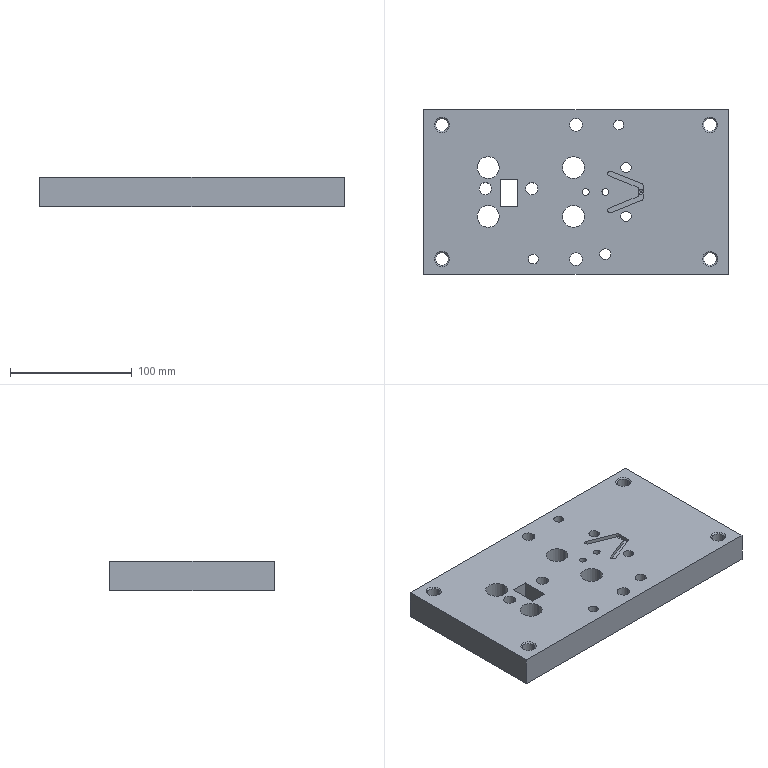Part | STEP file | MIENG DE KHUON DUONG KO LOGO | 1 solid | 120 faces | box 250 x 135 x 24 mm | volume 743044 mm3 | cylinder 67 | plane 31 | cone 22 | commonest cylinder face diameters 10.5 x12 4 x8 10 x8 18 x8 8 x6 13.5 x6